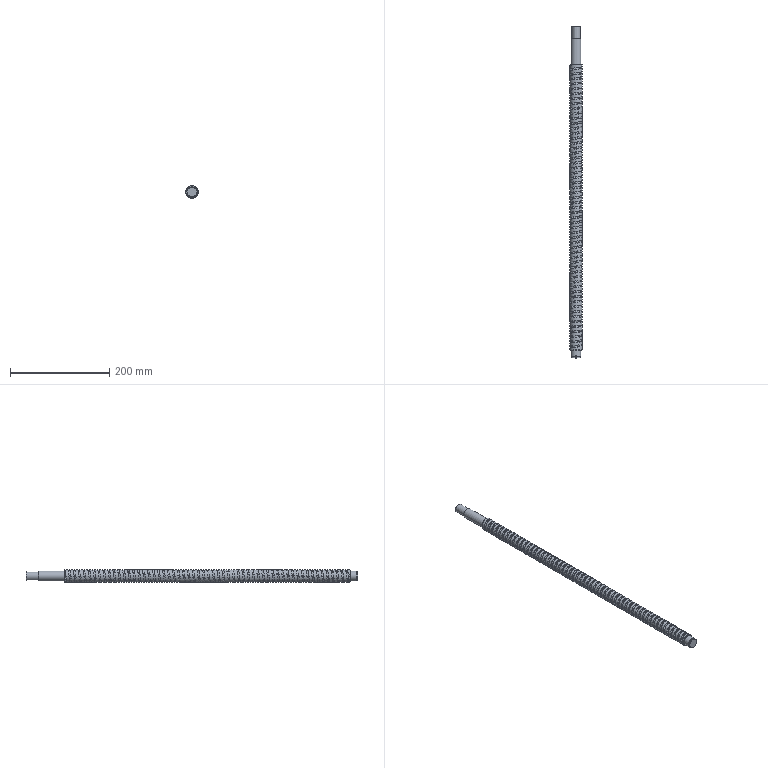Part | STEP file | 25 lead screw BK_id1386_x_t | 1 solid | 22 faces | box 25 x 669.5 x 25 mm | volume 331480 mm3 | plane 8 | cylinder 6 | cone 5 | spline 3 | commonest cylinder face diameters 20 x3 17 x1 19.2 x1 25 x1